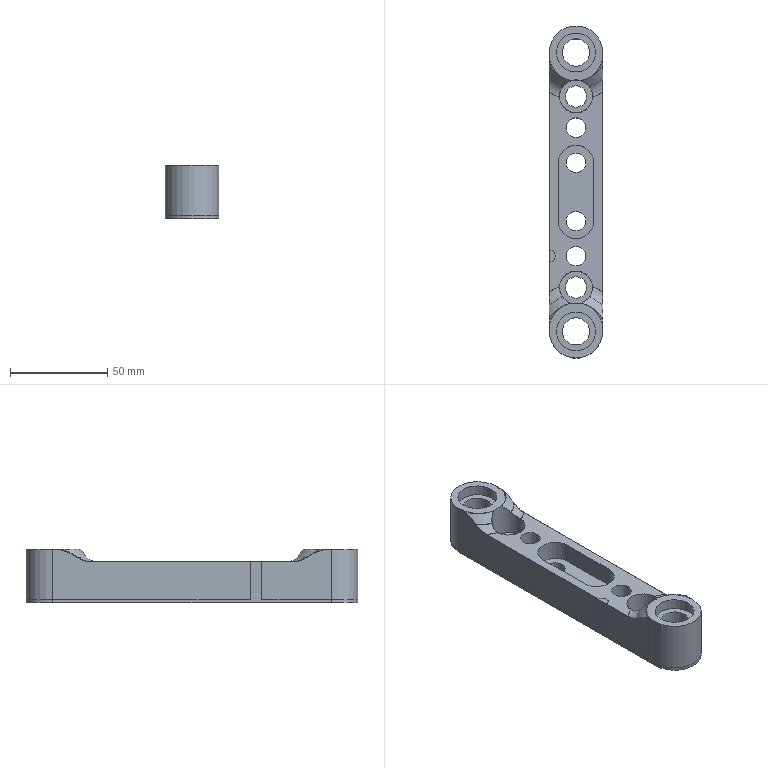NC program | NX | posted with a generic post | part box 27.4 x 170.48 x 27.5 mm
Lines 86 to 902 of 10888:
(ADAPTIVE_MILLING , TOOL : D12开粗)
N140 T05 M6
N142 G54
N144 G17 G0 G90 X0.8 Y-27.099 B0. C0. S4000 M3
N146 G43 Z30. H5
N148 Z-12.
N150 G94 G1 Y-26.949 Z-12.937 F1500.
N152 Y-26.799 Z-13.308
N154 X0.801 Y-26.649 Z-13.58
N156 Y-26.499 Z-13.8
N158 Y-26.349 Z-13.984
N160 Y-26.199 Z-14.142
N162 X0.802 Y-26.049 Z-14.28
N164 Y-25.899 Z-14.4
N166 Y-25.749 Z-14.505
N168 Y-25.599 Z-14.598
N170 X0.803 Y-25.449 Z-14.679
N172 Y-25.299 Z-14.75
N174 Y-25.149 Z-14.81
N176 Y-24.999 Z-14.862
N178 X0.804 Y-24.849 Z-14.905
N180 Y-24.699 Z-14.939
N182 Y-24.549 Z-14.966
N184 X0.805 Y-24.399 Z-14.985
N186 Y-24.249 Z-14.996
N188 Y-24.099 Z-15.
N190 X0.808 Y-22.225
N192 G3 X-0.004 Y-21.078 R1.212
N194 X-2.727 Y-20.673 R10.913
N196 X-12.398 Y-20.543 R185.874
N198 G1 X-23.462 Y-20.544
N200 X-35.649 Y-20.543
N202 X-47.899 Y-20.544
N204 X-60.087 Y-20.543
N206 X-67.242 Y-20.529
N208 X-87.741 Y-20.528
N210 G2 X-92.595 Y-18.16 R6.632
N212 X-94.893 Y-13.297 R10.684
N214 X-95.454 Y-7.645 R31.382
N216 X-95.526 Y3.417 R509.26
N218 X-95.51 Y13.112 R533.147
N220 X-92.872 Y17.834 R6.798
N222 X-87.991 Y19.956 R11.157
N224 X-81.958 Y20.474 R35.853
N226 X-71.52 Y20.528 R695.657
N228 G1 X87.656 Y20.529
N230 G2 X92.536 Y18.217 R6.6
N232 X94.828 Y13.556 R10.471
N234 X95.442 Y7.974 R28.891
N236 X95.526 Y-3.401 R426.377
N238 X95.511 Y-13.108 R533.408
N240 X92.873 Y-17.829 R6.8
N242 X87.992 Y-19.953 R11.167
N244 X82.022 Y-20.472 R35.405
N246 X71.512 Y-20.528 R693.764
N248 G1 X-56.876 Y-20.529
N250 G3 X-61.121 Y-20.112 R23.585
N252 X-72.367 Y-20.03 R444.916
N254 G1 X-85.429 Y-20.029
N256 G2 X-92.339 Y-16.249 R8.465
N258 X-94.432 Y-10.872 R13.606
N260 X-94.969 Y-4.213 R42.895
N262 X-95.01 Y10.862 R788.011
N264 X-91.15 Y17.404 R8.503
N266 X-85.681 Y19.466 R13.867
N268 X-78.956 Y19.975 R45.246
N270 X-67.415 Y20.028 R740.197
N272 G1 X85.356
N274 G2 X92.278 Y16.328 R8.459
N276 X94.413 Y10.956 R13.483
N278 X94.96 Y4.549 R40.869
N280 X95.01 Y-10.857 R704.877
N282 X91.216 Y-17.357 R8.502
N284 X85.946 Y-19.416 R13.589
N286 X79.539 Y-19.962 R40.795
N288 X67.405 Y-20.028 R710.24
N290 G1 X-58.041 Y-20.029
N292 X-58.312 Y-20.
N294 X-62.365
N296 X-71.54
N298 G2 X-74.961 Y-19.733 R28.927
N300 G3 X-82.324 Y-19.539 R98.637
N302 G2 X-85.862 Y-19.266 R15.227
N304 X-92.147 Y-14.437 R9.787
N306 X-94.005 Y-8.696 R16.445
N308 X-94.482 Y-1.342 R56.533
N310 X-94.499 Y9.157 R311.386
N312 X-89.666 Y17.009 R9.662
N314 X-84.021 Y18.953 R15.846
N316 X-77.046 Y19.468 R50.214
N318 G1 X-75.86 Y19.509
N320 G2 X-71.54 Y20. R17.863
N322 G1 X71.54
N324 G2 X74.956 Y19.733 R28.658
N326 G3 X82.377 Y19.537 R98.846
N328 G2 X86.036 Y19.222 R14.412
N330 X92.139 Y14.442 R9.808
N332 X94.001 Y8.707 R16.428
N334 X94.481 Y1.353 R56.276
N336 X94.503 Y-9.084 R366.937
N338 X89.687 Y-16.993 R9.666
N340 X83.804 Y-18.987 R16.06
N342 X76.514 Y-19.478 R54.488
N344 G3 X75.426 Y-19.619 R3.016
N346 G2 X71.54 Y-20. R20.544
N348 G1 X35.839
N350 G2 X33.959 Y-19.777 R15.888
N352 G3 X31.907 Y-19.657 R12.895
N354 G2 X29.839 Y-20. R7.185
N356 G1 X-62.335
N358 X-71.54
N360 G2 X-76.217 Y-19.439 R20.399
N362 G3 X-80.763 Y-19.098 R33.932
N364 G2 X-84.722 Y-18.732 R18.524
N366 X-91.587 Y-13.371 R10.609
N368 X-93.505 Y-7.193 R17.99
N370 X-93.985 Y0.725 R63.796
N372 X-93.988 Y7.662 R158.349
N374 X-88.505 Y16.505 R10.533
N376 X-82.414 Y18.471 R17.496
N378 X-78.067 Y18.891 R63.352
N380 X-75.836 Y19.515 R19.071
N382 G3 X-74.974 Y20.996 R1.2
N384 X-75.734 Y21.816 Z-14.951 R1.247
N386 G1 X-76.846 Y22.323 Z-14.9
N388 X-78.837 Y23.232 F15000.
N390 G3 X-79.627 Y23.305 R1.205
N392 G1 X-81.484 Y22.844
N394 X-83.336 Y22.367
N396 G3 X-88.81 Y20.357 R37.129
N398 X-93.007 Y17.791 R18.331
N400 X-95.457 Y14.772 R10.369
N402 G1 X-96.106 Y13.572
N404 X-96.739 Y12.365
N406 G3 X-97.82 Y9.093 R12.366
N408 X-97.966 Y7.13 R10.457
N410 G1 X-97.795 Y-1.058
N412 G3 X-96.913 Y-9.173 R48.258
N414 X-94.716 Y-15.258 R19.578
N416 X-91.368 Y-19.331 R15.68
N418 G1 X-90.648 Y-19.958
N420 X-89.918 Y-20.573
N422 G3 X-87.269 Y-21.998 R9.033
N424 X-84.872 Y-22.576 R12.553
N426 G1 X-79.639 Y-23.302
N428 G3 X-78.999 Y-23.215 R1.212
N430 G1 X-76.938 Y-22.324
N432 X-76.264 Y-22.036 Z-14.931 F1500.
N434 X-75.595 Y-21.738 Z-14.962
N436 G3 X-75.009 Y-21.063 Z-15. R1.2
N438 X-75.849 Y-19.511 R1.2
N440 X-80.939 Y-18.67 R21.923
N442 G2 X-86.168 Y-17.321 R13.407
N444 X-91.475 Y-11.524 R11.875
N446 X-93.09 Y-5.187 R21.424
N448 X-93.495 Y3.299 R82.459
N450 X-93.332 Y7.729 R28.414
N452 X-87.51 Y15.965 R11.141
N454 X-81.222 Y17.949 R18.636
N456 G3 X-79.815 Y18.189 R8.47
N458 G2 X-77.93 Y18.931 R16.33
N460 G3 X-77.514 Y20.921 R1.2
N462 X-78.338 Y21.262 Z-14.962 R1.277
N464 G1 X-79.801 Y21.408 Z-14.9
N466 X-82.149 Y21.644 F15000.
N468 X-82.362 Y21.645
N470 X-82.572 Y21.611
N472 X-83.923 Y21.261
N474 X-85.27 Y20.896
N476 G3 X-88.816 Y19.355 R16.145
N478 X-92.834 Y16.485 R26.881
N480 X-95.945 Y12.131 R12.085
N482 X-96.678 Y9.296 R10.901
N484 X-97.177 Y2.637 R64.494
N486 X-97.205 Y-0.636 R71.68
N488 X-96.405 Y-7.699 R40.063
N490 G1 X-96.12 Y-9.104
N492 X-95.819 Y-10.506
N494 G3 X-93.976 Y-15.04 R16.494
N496 X-91.102 Y-18.385 R13.878
N498 X-88.36 Y-20.259 R15.666
N500 X-84.781 Y-21.88 R22.516
N502 G1 X-84.151 Y-22.084
N504 X-83.515 Y-22.272
N506 X-81.268 Y-22.888
N508 G3 X-80.42 Y-22.807 R1.204
N510 G1 X-78.563 Y-21.891
N512 X-77.299 Y-21.263 Z-14.959 F1500.
N514 G3 X-76.729 Y-20.51 Z-15. R1.2
N516 X-77.478 Y-19.098 R1.2
N518 X-79.876 Y-18.446 R10.675
N520 G2 X-84.15 Y-17.378 R20.55
N522 X-90.78 Y-10.96 R12.394
N524 X-92.527 Y-4.463 R21.63
N526 X-92.922 Y5.456 R65.518
N528 X-89.841 Y12.939 R11.811
N530 X-83.781 Y16.604 R13.922
N532 G1 X-81.755 Y17.183
N534 G2 X-79.779 Y18.207 R21.813
N536 G3 X-79.301 Y19.929 R1.2
N538 X-80.236 Y20.485 Z-14.953 R1.255
N540 G1 X-81.476 Y20.681 Z-14.9
N542 X-83.646 Y21.025 F15000.
N544 G3 X-84.421 Y20.887 R1.206
N546 G1 X-87.007 Y19.425
N548 G3 X-90.081 Y17.356 R32.339
N550 G1 X-91.654 Y16.151
N552 X-92.176 Y15.713
N554 X-92.676 Y15.25
N556 G3 X-93.389 Y14.398 R7.049
N558 G1 X-93.978 Y13.564
N560 X-94.558 Y12.722
N562 G3 X-96.515 Y8.294 R14.849
N564 X-96.876 Y4.887 R12.484
N566 G1 X-96.803 Y2.532
N568 X-96.713 Y0.177
N570 G3 X-95.637 Y-7.658 R47.611
N572 G1 X-95.343 Y-8.989
N574 X-95.033 Y-10.317
N576 G3 X-93.395 Y-13.849 R11.401
N578 X-90.615 Y-17.319 R32.066
N580 G1 X-88.969 Y-19.102
N582 G3 X-85.111 Y-21.161 R6.643
N584 G1 X-82.824 Y-21.518
N586 X-82.677 Y-21.529
N588 X-82.529 Y-21.527
N590 X-80.12 Y-21.307
N592 X-78.415 Y-21.147 Z-14.972 F1500.
N594 G3 X-77.814 Y-20.872 Z-15. R1.205
N596 X-78.182 Y-18.838 R1.2
N598 X-82.071 Y-17.521 R72.14
N600 G2 X-90.461 Y-9.648 R13.584
N602 X-92.096 Y-2.737 R24.598
N604 X-92.357 Y4.625 R46.182
N606 X-89.005 Y12.442 R12.183
N608 X-83.922 Y15.722 R14.642
N610 G3 X-83.132 Y16.298 R3.956
N612 G1 X-81.654 Y17.236
N614 G3 X-81.819 Y19.35 R1.2
N616 X-82.6 Y19.416 Z-14.967 R1.291
N618 G1 X-84.166 Y19.163 Z-14.9
N620 X-86.357 Y18.809 F15000.
N622 G3 X-86.832 Y18.623 R1.232
N624 G1 X-89.929 Y16.558
N626 G3 X-94.456 Y11.057 R12.286
N628 X-95.427 Y8.46 R24.925
N630 X-96.281 Y1.782 R20.257
N632 X-95.64 Y-4.491 R42.078
N634 X-94.776 Y-8.255 R42.14
N636 X-92.991 Y-12.651 R23.57
N638 X-92.044 Y-14.353 R25.055
N640 X-89.045 Y-17.811 R15.474
N642 X-86.469 Y-19.656 R17.519
N644 G1 X-84.106 Y-21.044
N646 G3 X-83.305 Y-21.193 R1.205
N648 G1 X-81.187 Y-20.848
N650 X-80.455 Y-20.731 Z-14.931 F1500.
N652 X-79.724 Y-20.604 Z-14.962
N654 G3 X-79.001 Y-20.108 Z-15. R1.2
N656 X-79.463 Y-18.363 R1.2
N658 G2 X-83.466 Y-16.343 R94.439
N660 X-90.203 Y-8.186 R15.048
N662 X-91.651 Y-1.101 R28.301
N664 X-91.692 Y4.638 R27.363
N666 X-86.214 Y13.581 R12.414
N668 G1 X-84.786 Y14.984
N670 X-83.661 Y15.878
N672 G3 X-83.591 Y17.698 R1.2
N674 X-84.616 Y18.005 Z-14.954 R1.258
N676 G1 X-85.887 Y17.906 Z-14.9
N678 X-87.972 Y17.742 F15000.
N680 G3 X-88.838 Y17.266 R1.202
N682 G1 X-92.412 Y12.501
N684 G3 X-94.563 Y8.619 R15.88
N686 X-95.192 Y6.483 R19.616
N688 X-95.62 Y2.09 R14.42
N690 G1 X-95.472 Y-0.322
N692 G3 X-94.106 Y-7.78 R38.728
N694 X-91.76 Y-13.223 R24.149
N696 G1 X-91.346 Y-13.929
N698 X-90.923 Y-14.629
N700 G3 X-88.298 Y-17.468 R11.246
N702 G1 X-86.538 Y-18.811
N704 G3 X-85.99 Y-19.043 R1.217
N706 G1 X-83.872 Y-19.365
N708 X-82.987 Y-19.504 Z-14.938 F1500.
N710 X-82.1 Y-19.629 Z-14.975
N712 G3 X-81.523 Y-19.536 Z-15. R1.206
N714 X-81.36 Y-17.423 R1.2
N716 G1 X-83.146 Y-16.288
N718 X-84.803 Y-14.97
N720 X-86.311 Y-13.484
N722 X-87.653 Y-11.847
N724 X-88.815 Y-10.078
N726 X-89.784 Y-8.196
N728 X-90.548 Y-6.222
N730 X-91.099 Y-4.178
N732 X-91.431 Y-2.087
N734 X-91.54 Y0.027
N736 G2 X-91.03 Y4.866 R29.477
N738 X-89.262 Y9.209 R13.172
N740 G1 X-88.798 Y10.107
N742 X-87.635 Y11.872
N744 X-86.204 Y13.591
N746 G3 X-86.662 Y15.584 R1.2
N748 X-87.6 Y15.517 Z-14.96 R1.276
N750 G1 X-88.917 Y14.991 Z-14.9
N752 X-90.926 Y14.189 F15000.
N754 G3 X-91.564 Y13.591 R1.203
N756 G1 X-95.216 Y5.927
N758 G3 X-95.208 Y4.88 R1.201
N760 G1 X-94.306 Y3.051
N762 X-93.98 Y2.386 Z-14.931 F1500.
N764 X-93.645 Y1.726 Z-14.962
N766 G3 X-92.957 Y1.179 Z-15. R1.2
N768 X-91.425 Y2.137 R1.2
N770 G1 X-91.089 Y4.223
N772 X-90.535 Y6.261
N774 X-89.768 Y8.23
N776 X-89.252 Y9.23
N778 G3 X-90.245 Y10.978 R1.2
N780 X-91.112 Y10.687 Z-14.961 R1.273
N782 G1 X-92.283 Y9.839 Z-14.9
N784 X-93.947 Y8.634 F15000.
N786 G3 X-94.429 Y7.842 R1.202
N788 G1 X-95.099 Y3.426
N790 G3 X-95.104 Y-2.463 R19.767
N792 X-94.374 Y-6.102 R27.644
N794 X-91.68 Y-12.183 R22.572
N796 X-89.136 Y-15.708 R31.306
N798 X-86.388 Y-18.338 R18.764
N800 G1 X-85.314 Y-19.179
N802 X-84.231 Y-20.007
N804 G3 X-81.566 Y-21.512 R13.974
N806 X-79.335 Y-22.327 R19.343
N808 X-76.77 Y-22.996 R26.027
N810 X-74.252 Y-23.337 R21.039
N812 X-67.571 Y-23.613 R84.132
N814 G1 X30.941 Y-23.679
N816 G3 X31.387 Y-23.594 R1.267
N818 G1 X33.603 Y-22.708
N820 X35.002 Y-22.144 Z-14.963 F1500.
N822 G3 X35.592 Y-21.527 Z-15. R1.2
N824 X34.731 Y-19.889 R1.2
N826 G2 X33.37 Y-19.544 R18.211
N828 G3 X32.283 Y-19.501 R2.225
N830 G1 X31.695 Y-19.712
N832 G3 X32.15 Y-22.274 R1.32
N834 G1 X33.519 Y-22.263
N836 G3 X33.952 Y-19.7 R1.32
N838 X32.84 Y-19.4 R3.544
N840 X32.328 Y-19.488 R7.463
N842 X31.453 Y-20.607 R1.2
N844 X31.899 Y-21.585 Z-14.953 R1.257
N846 G1 X32.81 Y-22.471 Z-14.9
N848 X34.167 Y-23.791 F15000.
N850 G3 X35.008 Y-24.131 R1.203
N852 G1 X60.314 Y-24.03
N854 G3 X78.144 Y-23.178 R204.137
N856 G1 X84.817 Y-22.566
N858 G3 X92.412 Y-19.508 R14.173
N860 G1 X93.629 Y-18.462
N862 X94.827 Y-17.394
N864 G3 X96.569 Y-14.96 R8.578
N866 X97.389 Y-12.648 R10.938
N868 G1 X97.724 Y-11.201
N870 X98.024 Y-9.747
N872 G3 X98.373 Y-7.096 R23.822
N874 X98.391 Y-5.314 R17.721
N876 G1 X97.853 Y7.33
N878 G3 X96.916 Y12.416 R18.937
N880 X95.236 Y16.329 R22.95
N882 X88.743 Y22.098 R13.255
N884 X84.997 Y23.003 R12.752
N886 G1 X78.182 Y23.584
N888 G3 X77.632 Y23.502 R1.222
N890 G1 X75.484 Y22.637
N892 X74.061 Y22.059 Z-14.965 F1500.
N894 G3 X73.482 Y21.468 Z-15. R1.201
N896 X74.392 Y19.794 R1.2
N898 G2 X76.592 Y19.38 R119.975
N900 G3 X81.864 Y19.069 R47.371
N902 G2 X87.331 Y17.726 R11.613
N904 X92.112 Y12.309 R11.31
N906 X93.631 Y6.198 R20.709
N908 X94.002 Y-2.165 R84.566
N910 X93.975 Y-7.852 R103.013
N912 X88.484 Y-16.515 R10.522
N914 X82.566 Y-18.447 R17.382
N916 X78.121 Y-18.88 R48.358
N918 X75.875 Y-19.508 R20.951
N920 G3 X75.006 Y-20.997 R1.2
N922 X75.767 Y-21.812 Z-14.952 R1.247
N924 G1 X76.883 Y-22.319 Z-14.9
N926 X78.877 Y-23.227 F15000.
N928 G3 X79.665 Y-23.299 R1.205
N930 G1 X81.522 Y-22.837
N932 X83.375 Y-22.36
N934 G3 X88.848 Y-20.35 R37.129
N936 X93.046 Y-17.784 R18.331
N938 X95.495 Y-14.765 R10.369
N940 X97.336 Y-10.123 R21.54
N942 X97.793 Y-6.283 R14.662
N944 G1 X97.669 Y2.65
N946 G3 X96.698 Y9.979 R31.476
N948 G1 X96.437 Y11.008
N950 X96.163 Y12.034
N952 G3 X94.476 Y15.978 R17.865
N954 X91.527 Y19.315 R11.996
N956 X84.526 Y22.51 R16.331
N958 G1 X83.979 Y22.607
N960 X79.641 Y23.305
N962 G3 X78.972 Y23.22 R1.211
N964 G1 X76.929 Y22.332
N966 X76.255 Y22.042 Z-14.931 F1500.
N968 X75.585 Y21.742 Z-14.962
N970 G3 X75.002 Y21.068 Z-15. R1.2
N972 X75.85 Y19.514 R1.2
N974 X80.936 Y18.671 R22.763
N976 G2 X86.109 Y17.349 R13.471
N978 X91.425 Y11.627 R11.837
N980 X93.09 Y5.177 R21.292
N982 X93.493 Y-3.185 R81.664
N984 X93.348 Y-7.615 R30.236
N986 X87.499 Y-15.969 R11.144
N988 X81.272 Y-17.939 R18.566
N990 G3 X79.835 Y-18.176 R11.321
N992 G2 X77.942 Y-18.926 R12.356
N994 G3 X77.543 Y-20.961 R1.2
N996 X78.335 Y-21.265 Z-14.964 R1.285
N998 G1 X79.845 Y-21.413 Z-14.9
N1000 X82.165 Y-21.639 F15000.
N1002 X82.376 Y-21.64
N1004 X82.584 Y-21.606
N1006 X83.936 Y-21.256
N1008 X85.283 Y-20.891
N1010 G3 X88.829 Y-19.35 R16.145
N1012 X92.846 Y-16.48 R26.881
N1014 X96.14 Y-11.669 R12.112
N1016 X96.725 Y-9.299 R11.363
N1018 X97.079 Y-4.861 R41.453
N1020 G1 X97.15 Y-2.215
N1022 X97.204 Y0.432
N1024 G3 X96.549 Y6.978 R32.892
N1026 X95.649 Y10.574 R29.714
N1028 X94.272 Y14.016 R29.714
N1030 X90.987 Y18.412 R13.04
N1032 X87.951 Y20.482 R15.336
N1034 X83.388 Y22.315 R21.589
N1036 G1 X81.001 Y22.969
N1038 G3 X80.159 Y22.891 R1.204
N1040 G1 X78.282 Y21.978
N1042 X77.014 Y21.355 Z-14.959 F1500.
N1044 G3 X76.441 Y20.608 Z-15. R1.2
N1046 X77.211 Y19.179 R1.2
N1048 X80.772 Y18.288 R16.455
N1050 G2 X86.093 Y16.39 R14.361
N1052 X91.126 Y10.162 R12.946
N1054 X92.626 Y3.603 R24.148
N1056 X92.922 Y-5.447 R66.501
N1058 X89.847 Y-12.93 R11.803
N1060 X83.683 Y-16.633 R13.972
N1062 G1 X81.744 Y-17.183
N1064 G2 X79.823 Y-18.181 R13.35
N1066 G3 X79.332 Y-19.958 R1.2
N1068 X80.254 Y-20.478 Z-14.954 R1.259
N1070 G1 X81.528 Y-20.672 Z-14.9
N1072 X83.698 Y-21.001 F15000.
N1074 G3 X84.465 Y-20.861 R1.206
N1076 G1 X87.051 Y-19.4
N1078 G3 X90.125 Y-17.331 R32.339
N1080 G1 X91.698 Y-16.125
N1082 X92.22 Y-15.687
N1084 X92.72 Y-15.225
N1086 G3 X93.433 Y-14.373 R7.049
N1088 G1 X94.022 Y-13.538
N1090 X94.602 Y-12.697
N1092 G3 X96.559 Y-8.269 R14.849
N1094 X96.92 Y-4.861 R12.484
N1096 G1 X96.835 Y-2.165
N1098 X96.734 Y0.531
N1100 G3 X95.372 Y8.887 R40.997
N1102 X93.599 Y13.349 R23.846
N1104 X92.647 Y15.088 R25.021
N1106 X88.898 Y19.112 R14.038
N1108 X86.994 Y20.233 R13.23
N1110 G1 X82.064 Y22.601
N1112 G3 X80.969 Y22.572 R1.201
N1114 G1 X79.263 Y21.639
N1116 X78.028 Y20.958 Z-14.959 F1500.
N1118 G3 X77.49 Y20.182 Z-15. R1.2
N1120 X78.274 Y18.811 R1.2
N1122 X82.063 Y17.522 R63.458
N1124 G2 X90.48 Y9.594 R13.596
N1126 X92.094 Y2.743 R24.686
N1128 X92.357 Y-4.62 R46.062
N1130 X88.999 Y-12.447 R12.186
N1132 X83.931 Y-15.718 R14.674
N1134 G3 X82.217 Y-16.911 R147.181
N1136 G1 X81.674 Y-17.22
N1138 G3 X81.837 Y-19.384 R1.2
N1140 X82.58 Y-19.428 Z-14.968 R1.312
N1142 G1 X84.185 Y-19.16 Z-14.9
N1144 X86.384 Y-18.793 F15000.
N1146 G3 X86.852 Y-18.608 R1.243
N1148 G1 X89.949 Y-16.543
N1150 G3 X94.476 Y-11.041 R12.286
N1152 X95.447 Y-8.445 R24.925
N1154 X96.301 Y-1.767 R20.257
N1156 X95.66 Y4.506 R42.078
N1158 X94.796 Y8.27 R42.14
N1160 X93.011 Y12.666 R23.57
N1162 X92.064 Y14.368 R25.055
N1164 X88.324 Y18.422 R15.506
N1166 X86.474 Y19.645 R16.776
N1168 G1 X83.817 Y21.155
N1170 G3 X83.043 Y21.298 R1.206
N1172 G1 X80.912 Y20.972
N1174 X79.412 Y20.737 Z-14.964 F1500.
N1176 G3 X78.703 Y20.278 Z-15. R1.201
N1178 X79.175 Y18.474 R1.2
N1180 G2 X84.079 Y15.982 R41.611
N1182 X90.252 Y8.044 R15.137
N1184 X91.669 Y0.89 R28.969
N1186 X91.664 Y-4.848 R26.054
N1188 X86.167 Y-13.612 R12.421
N1190 G1 X85.538 Y-14.284
N1192 G2 X83.795 Y-15.794 R33.481
N1194 G3 X83.69 Y-17.67 R1.2
N1196 X84.71 Y-17.959 Z-14.954 R1.259
N1198 G1 X85.992 Y-17.845 Z-14.9
N1200 X88.118 Y-17.657 F15000.
N1202 G3 X88.972 Y-17.182 R1.202
N1204 G1 X92.55 Y-12.412
N1206 G3 X93.973 Y-9.843 R10.732
N1208 X95.248 Y-5.774 R35.856
N1210 X95.608 Y-1.928 R13.85
N1212 G1 X95.55 Y-0.722
N1214 X95.483 Y0.484
N1216 G3 X94.134 Y8.009 R37.436
N1218 X91.806 Y13.288 R22.144
N1220 X90.588 Y15.112 R16.97
N1222 X87.951 Y17.648 R13.19
N1224 G1 X85.799 Y19.207
N1226 G3 X85.287 Y19.419 R1.223
N1228 G1 X83.274 Y19.745
N1230 X82.301 Y19.906 Z-14.941 F1500.
N1232 X81.325 Y20.054 Z-14.983
N1234 X81.121 Y20.057 Z-14.991
N1236 X80.92 Y20.026 Z-15.
N1238 G3 X80.621 Y17.819 R1.2
N1240 G1 X82.219 Y16.911
N1242 X83.949 Y15.685
N1244 X85.54 Y14.283
N1246 X86.973 Y12.721
N1248 X88.233 Y11.016
N1250 X89.305 Y9.187
N1252 X90.178 Y7.254
N1254 X90.841 Y5.24
N1256 X91.288 Y3.168
N1258 X91.512 Y1.059
N1260 G2 X91.051 Y-4.745 R25.765
N1262 X89.374 Y-9.033 R13.337
N1264 X88.232 Y-11.017 R56.762
N1266 G1 X86.972 Y-12.722
N1268 X86.085 Y-13.689
N1270 G3 X86.597 Y-15.642 R1.2
N1272 X87.502 Y-15.581 Z-14.961 R1.274
N1274 G1 X88.86 Y-15.061 Z-14.9
N1276 X90.775 Y-14.328 F15000.
N1278 G3 X91.445 Y-13.689 R1.203
N1280 G1 X95.295 Y-4.913
N1282 G3 X95.282 Y-3.92 R1.202
N1284 G1 X94.409 Y-2.066
N1286 X93.747 Y-0.672 Z-14.965 F1500.
N1288 G3 X93.13 Y-0.13 Z-15. R1.201
N1290 X91.505 Y-1.123 R1.2
N1292 G1 X91.287 Y-3.169
N1294 X90.841 Y-5.242
N1296 X90.177 Y-7.256
N1298 X89.354 Y-9.078
N1300 G3 X89.675 Y-10.502 R1.212
N1302 G1 X91.219 Y-11.811
N1304 X91.333 Y-11.908 Z-14.996
N1306 X91.447 Y-12.005 Z-14.985
N1308 X91.562 Y-12.102 Z-14.966
N1310 X91.676 Y-12.199 Z-14.939
N1312 X91.791 Y-12.296 Z-14.905
N1314 X91.905 Y-12.393 Z-14.862
N1316 X92.019 Y-12.49 Z-14.81
N1318 X92.134 Y-12.587 Z-14.75
N1320 X92.248 Y-12.684 Z-14.679
N1322 X92.363 Y-12.781 Z-14.598
N1324 X92.477 Y-12.878 Z-14.505
N1326 X92.591 Y-12.975 Z-14.4
N1328 X92.706 Y-13.072 Z-14.28
N1330 X92.82 Y-13.169 Z-14.142
N1332 X92.935 Y-13.266 Z-13.984
N1334 X93.049 Y-13.363 Z-13.8
N1336 X93.163 Y-13.46 Z-13.58
N1338 X93.278 Y-13.557 Z-13.308
N1340 X93.392 Y-13.654 Z-12.937
N1342 X93.507 Y-13.751 Z-12.
N1344 G0 Z30.
N1346 X55.914 Y-25.851
N1348 Z-3.199
N1350 G1 X55.957 Y-25.707 Z-4.136
N1352 X56. Y-25.564 Z-4.507
N1354 X56.043 Y-25.42 Z-4.779
N1356 X56.086 Y-25.276 Z-4.999
N1358 X56.13 Y-25.133 Z-5.183
N1360 X56.173 Y-24.989 Z-5.341
N1362 X56.216 Y-24.845 Z-5.479
N1364 X56.259 Y-24.702 Z-5.599
N1366 X56.302 Y-24.558 Z-5.704
N1368 X56.345 Y-24.414 Z-5.797
N1370 X56.388 Y-24.271 Z-5.878
N1372 X56.432 Y-24.127 Z-5.949
N1374 X56.475 Y-23.984 Z-6.009
N1376 X56.518 Y-23.84 Z-6.061
N1378 X56.561 Y-23.696 Z-6.104
N1380 X56.604 Y-23.553 Z-6.138
N1382 X56.647 Y-23.409 Z-6.165
N1384 X56.69 Y-23.265 Z-6.184
N1386 X56.734 Y-23.122 Z-6.195
N1388 X56.777 Y-22.978 Z-6.199
N1390 X57.171 Y-21.665
N1392 G3 X55.542 Y-20.198 R1.212
N1394 G2 X51.926 Y-20.371 R5.627
N1396 G3 X49.262 Y-19.775 R27.005
N1398 X43.176 Y-19.516 R57.883
N1400 G2 X37.343 Y-19.47 R297.339
N1402 X34.185 Y-19.101 R120.454
N1404 G3 X32.329 Y-19.214 R8.94
N1406 G2 X25.149 Y-19.481 R78.565
N1408 G1 X17.899 Y-19.494
N1410 X-46.31 Y-19.5
N1412 G3 X-48.464 Y-19.867 R5.081
N1414 G2 X-52.475 Y-19.916 R7.655
N1416 X-56.076 Y-20. R41.388
N1418 G3 X-57.396 Y-21.32 R1.32
N1420 X-56.076 Y-22.64 R1.32
N1422 G1 X-52.804
N1424 X-50.421 Z-6.099
N1426 X50.526 F15000.
N1428 X52.909 Z-6.199 F1500.
N1430 X55.818
N1432 G3 X57.138 Y-21.32 R1.32
N1434 X55.818 Y-20. R1.32
N1436 G2 X52.356 Y-19.915 R37.321
N1438 G3 X48.755 Y-19.338 R125.11
N1440 X41.421 Y-19.02 R75.469
N1442 G2 X35.597 Y-18.733 R57.475
N1444 G3 X32.407 Y-18.771 R28.97
N1446 G2 X19.035 Y-18.992 R272.421
N1448 G1 X-43.836 Y-18.999
N1450 G3 X-47.886 Y-19.3 R19.596
N1452 G1 X-49.693 Y-19.421
N1454 X-49.933 Y-19.492
N1456 G3 X-50.507 Y-21.342 R1.32
N1458 X-49.255 Y-22.003 Z-6.136 R1.356
N1460 G1 X-48.364 Y-22.005 Z-6.099
N1462 X48.901 Y-22.246 F15000.
N1464 X50.465 Z-6.165 F1500.
N1466 G3 X51.217 Y-21.962 Z-6.199 R1.323
N1468 X50.74 Y-19.656 R1.32
N1470 X47.302 Y-18.876 R22.791
N1472 X40.841 Y-18.53 R68.113
N1474 X35.668 Y-18.275 R855.101
N1476 X27.753 Y-18.425 R278.219
N1478 G2 X14.629 Y-18.494 R772.823
N1480 G1 X-42.758 Y-18.499
N1482 G3 X-47.446 Y-18.749 R51.628
N1484 X-49.111 Y-18.991 R7.431
N1486 G1 X-50.009 Y-19.529
N1488 X-50.265 Y-19.611
N1490 G2 X-52.63 Y-19.912 R25.434
N1492 G3 X-52.534 Y-22.549 R1.32
N1494 G1 X-52.044 Y-22.545
N1496 X-49.662 Y-22.523 Z-6.099
N1498 X47.381 Y-21.626 F15000.
N1500 X48.483 Y-21.61 Z-6.145 F1500.
N1502 G3 X49.527 Y-20.96 Z-6.199 R1.319
N1504 X49.161 Y-19.228 R1.32
N1506 X46.669 Y-18.494 R7.655
N1508 X41.513 Y-18.074 R49.82
N1510 X29.586 Y-17.887 R115.137
N1512 G2 X14.462 Y-17.993 R782.589
N1514 G1 X-41.319 Y-17.999
N1516 G3 X-47.773 Y-18.353 R50.054
N1518 X-48.409 Y-18.535 R2.377
N1520 G1 X-49.258 Y-19.063
N1522 G3 X-49.702 Y-20.846 R1.32
N1524 X-48.451 Y-21.504 Z-6.137 R1.356
N1526 G1 X-47.558 Y-21.505 Z-6.099
N1528 X47.374 Y-21.619 F15000.
N1530 X48.475 Y-21.615 Z-6.145 F1500.
N1532 G3 X49.526 Y-20.976 Z-6.199 R1.319
N1534 X49.161 Y-19.228 R1.32
N1536 X46.861 Y-18.254 R5.756
N1538 X41.766 Y-17.629 R33.987
N1540 X30.622 Y-17.375 R111.394
N1542 G2 X13.625 Y-17.493 R836.481
N1544 G1 X-40.129 Y-17.499
N1546 G3 X-46.705 Y-17.798 R58.616
N1548 X-47.579 Y-18.019 R2.705
N1550 G1 X-48.428 Y-18.547
N1552 G3 X-48.876 Y-20.326 R1.32
N1554 X-47.626 Y-20.988 Z-6.137 R1.356
N1556 G1 X-46.733 Y-20.992 Z-6.099
N1558 X47.065 Y-21.397 F15000.
N1560 X48.166 Z-6.145 F1500.
N1562 G3 X49.219 Y-20.761 Z-6.199 R1.319
N1564 X48.857 Y-19.009 R1.32
N1566 X46.37 Y-17.869 R6.239
N1568 X40.914 Y-17.117 R34.402
N1570 X30.539 Y-16.886 R114.338
N1572 G2 X11.983 Y-16.993 R925.118
N1574 G1 X-38.758 Y-16.998
N1576 G3 X-45.625 Y-17.251 R70.9
N1578 X-46.798 Y-17.534 R2.987
N1580 G1 X-47.6 Y-18.032
N1582 G3 X-48.048 Y-19.808 R1.32
N1584 X-46.8 Y-20.473 Z-6.136 R1.356
N1586 G1 X-45.908 Y-20.479 Z-6.099
N1588 X46.605 Y-21.067 F15000.
N1590 X47.707 Y-21.069 Z-6.145 F1500.
N1592 G3 X48.76 Y-20.435 Z-6.199 R1.319
N1594 X48.4 Y-18.681 R1.32
N1596 X45.667 Y-17.415 R6.829
N1598 X39.421 Y-16.566 R35.4
N1600 X28.409 Y-16.415 R150.946
N1602 G2 X11.034 Y-16.493 R957.69
N1604 G1 X-37.14 Y-16.497
N1606 G3 X-44.522 Y-16.709 R88.832
N1608 X-46.351 Y-17.115 R5.441
N1610 G1 X-46.554 Y-17.26
N1612 G3 X-46.776 Y-18.906 R1.32
N1614 X-45.548 Y-19.541 Z-6.138 R1.36
N1616 G1 X-44.618 Y-19.553 Z-6.099
N1618 X46.038 Y-20.66 F15000.
N1620 X47.14 Y-20.668 Z-6.145 F1500.
N1622 G3 X48.198 Y-20.041 Z-6.199 R1.319
N1624 X47.841 Y-18.28 R1.32
N1626 X44.96 Y-16.942 R7.339
N1628 X38.627 Y-16.072 R34.077
N1630 X28.333 Y-15.92 R154.42
N1632 G2 X14.335 Y-15.99 R880.058
N1634 G1 X-35.457 Y-15.996
N1636 G3 X-43.563 Y-16.188 R106.911
N1638 X-45.864 Y-16.657 R7.946
N1640 X-46.514 Y-17.067 R1.975
N1642 X-46.592 Y-18.711 R1.32
N1644 X-45.422 Y-19.26 Z-6.142 R1.366
N1646 G1 X-44.388 Y-19.271 Z-6.099
N1648 X45.483 Y-20.26 F15000.
N1650 X46.584 Y-20.267 Z-6.145 F1500.
N1652 G3 X47.641 Y-19.637 Z-6.199 R1.319
N1654 X47.283 Y-17.879 R1.32
N1656 X44.171 Y-16.437 R7.881
N1658 X37.772 Y-15.578 R34.17
N1660 X27.635 Y-15.431 R166.463
N1662 G2 X12.638 Y-15.491 R964.038
N1664 G1 X-33.461 Y-15.495
N1666 G3 X-42.291 Y-15.644 R149.856
N1668 X-45.363 Y-16.176 R11.692
N1670 X-46.512 Y-16.89 R2.576
N1672 X-46.453 Y-18.522 R1.32
N1674 X-45.337 Y-18.988 Z-6.146 R1.367
N1676 G1 X-44.209 Y-18.991 Z-6.099
N1678 X44.325 Y-19.203 F15000.
N1680 X45.6 Y-19.201 Z-6.153 F1500.
N1682 G3 X46.553 Y-18.707 Z-6.199 R1.319
N1684 X46.788 Y-17.524 R1.321
N1686 X45.028 Y-16.44 R4.668
N1688 X40.011 Y-15.338 R20.214
N1690 X30.887 Y-14.936 R86.772
N1692 G1 X19.007 Y-14.979
N1694 X10.07 Y-14.991
N1696 X-34.698 Y-14.996
N1698 G3 X-42.284 Y-15.204 R92.746
N1700 X-45.449 Y-15.916 R10.184
N1702 X-46.637 Y-17.073 R2.108
N1704 G1 X-46.783 Y-17.524
N1706 X-46.836 Y-17.557
N1708 G3 X-47.28 Y-19.342 R1.32
N1710 X-46.018 Y-19.997 Z-6.136 R1.356
N1712 G1 X-45.135 Y-19.99 Z-6.099
N1714 X44.332 Y-19.217 F15000.
N1716 X45.614 Y-19.2 Z-6.153 F1500.
N1718 G3 X46.557 Y-18.701 Z-6.199 R1.319
N1720 X46.788 Y-17.524 R1.321
N1722 X45.286 Y-16.324 R3.681
N1724 X40.93 Y-15.067 R15.218
N1726 X32.563 Y-14.476 R61.487
N1728 X18.002 Y-14.481 R874.684
N1730 G1 X9.752 Y-14.491
N1732 X-33.7 Y-14.496
N1734 G3 X-41.397 Y-14.686 R104.212
N1736 X-45.016 Y-15.424 R12.644
N1738 X-46.06 Y-16.117 R2.259
N1740 G1 X-46.355 Y-16.596
N1742 G3 X-46.26 Y-18.117 R1.32
N1744 X-45.129 Y-18.609 Z-6.145 R1.365
N1746 G1 X-44.028 Y-18.615 Z-6.099
N1748 X44.232 Y-19.058 F15000.
N1750 X45.33 Z-6.145 F1500.
N1752 G3 X46.385 Y-18.42 Z-6.199 R1.319
N1754 X46.366 Y-17.037 R1.321
N1756 X44.802 Y-15.86 R4.136
N1758 X40.317 Y-14.584 R15.997
N1760 X31.932 Y-13.991 R62.86
N1762 X16.685 Y-13.983 R892.314
N1764 G1 X9.372 Y-13.991
N1766 X-32.826 Y-13.995